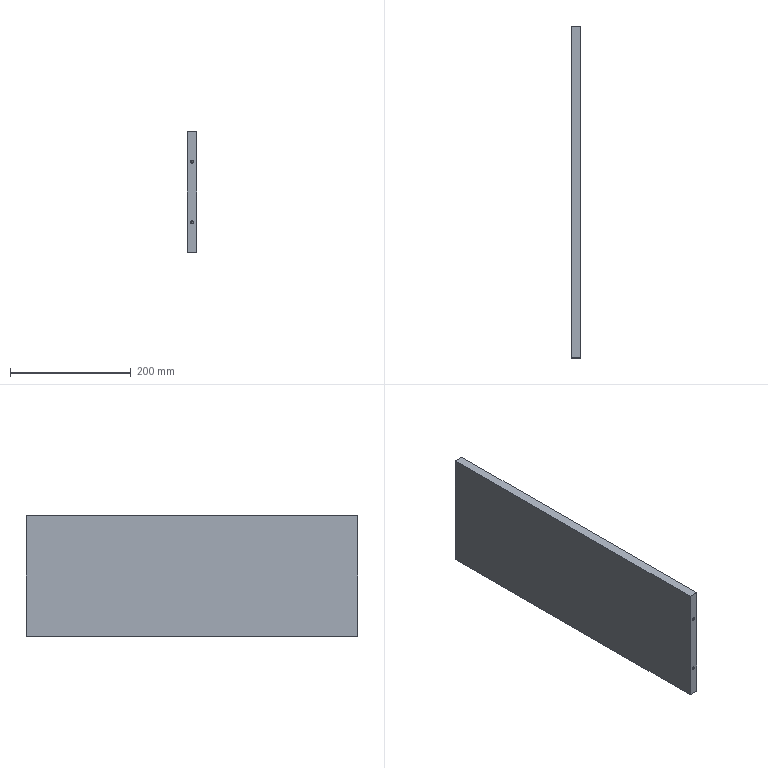Part | NX | features DATUM_CSYS 4, SIMPLE HOLE 4, SYMBOLIC_THREAD 4, SKETCH 3, EXTRACT_FACE 2, HOLE PACKAGE 2, EXTRUDE 1, Instance Feature 1, Mirror Feature 1 | 1 solid | 18 faces | box 15 x 550 x 200 mm | volume 1648864 mm3 | cone 8 | plane 6 | cylinder 4 | commonest cylinder face diameters 4.2 x4
STEP:
#1=CARTESIAN_POINT('',(-7.5,275.,0.));
#2=VERTEX_POINT('',#1);
#3=CARTESIAN_POINT('',(-7.5,-275.,0.));
#4=VERTEX_POINT('',#3);
#5=CARTESIAN_POINT('',(-7.5,275.,0.));
#6=DIRECTION('',(0.,-1.,0.));
#7=VECTOR('',#6,1000.);
#8=LINE('',#5,#7);
#9=EDGE_CURVE('',#2,#4,#8,.T.);
#10=ORIENTED_EDGE('',*,*,#9,.T.);
#11=CARTESIAN_POINT('',(-7.5,-275.,200.));
#12=VERTEX_POINT('',#11);
#13=CARTESIAN_POINT('',(-7.5,-275.,200.));
#14=DIRECTION('',(0.,0.,-1.));
#15=VECTOR('',#14,1000.);
#16=LINE('',#13,#15);
#17=EDGE_CURVE('',#12,#4,#16,.T.);
#18=ORIENTED_EDGE('',*,*,#17,.F.);
#19=CARTESIAN_POINT('',(-7.5,275.,200.));
#20=VERTEX_POINT('',#19);
#21=CARTESIAN_POINT('',(-7.5,275.,200.));
#22=DIRECTION('',(0.,-1.,0.));
#23=VECTOR('',#22,1000.);
#24=LINE('',#21,#23);
#25=EDGE_CURVE('',#20,#12,#24,.T.);
#26=ORIENTED_EDGE('',*,*,#25,.F.);
#27=CARTESIAN_POINT('',(-7.5,275.,200.));
#28=DIRECTION('',(0.,0.,-1.));
#29=VECTOR('',#28,1000.);
#30=LINE('',#27,#29);
#31=EDGE_CURVE('',#20,#2,#30,.T.);
#32=ORIENTED_EDGE('',*,*,#31,.T.);
#33=EDGE_LOOP('',(#10,#18,#26,#32));
#34=FACE_BOUND('',#33,.T.);
#35=CARTESIAN_POINT('',(-7.5,275.,200.));
#36=DIRECTION('',(1.,0.,0.));
#37=DIRECTION('',(0.,1.,0.));
#38=AXIS2_PLACEMENT_3D('',#35,#36,#37);
#39=PLANE('',#38);
#40=ADVANCED_FACE('',(#34),#39,.F.);
#41=CARTESIAN_POINT('',(0.,-275.,152.5));
#42=VERTEX_POINT('',#41);
#43=CARTESIAN_POINT('',(0.,-275.,150.));
#44=DIRECTION('',(0.,1.,0.));
#45=DIRECTION('',(0.,0.,1.));
#46=AXIS2_PLACEMENT_3D('',#43,#44,#45);
#47=CIRCLE('',#46,2.5);
#48=EDGE_CURVE('',#42,#42,#47,.T.);
#49=ORIENTED_EDGE('',*,*,#48,.T.);
#50=EDGE_LOOP('',(#49));
#51=FACE_BOUND('',#50,.T.);
#52=CARTESIAN_POINT('',(0.,-275.,52.5));
#53=VERTEX_POINT('',#52);
#54=CARTESIAN_POINT('',(0.,-275.,50.));
#55=DIRECTION('',(0.,1.,0.));
#56=DIRECTION('',(0.,0.,1.));
#57=AXIS2_PLACEMENT_3D('',#54,#55,#56);
#58=CIRCLE('',#57,2.5);
#59=EDGE_CURVE('',#53,#53,#58,.T.);
#60=ORIENTED_EDGE('',*,*,#59,.T.);
#61=EDGE_LOOP('',(#60));
#62=FACE_BOUND('',#61,.T.);
#63=CARTESIAN_POINT('',(7.5,-275.,0.));
#64=VERTEX_POINT('',#63);
#65=CARTESIAN_POINT('',(-7.5,-275.,0.));
#66=DIRECTION('',(1.,0.,0.));
#67=VECTOR('',#66,1000.);
#68=LINE('',#65,#67);
#69=EDGE_CURVE('',#4,#64,#68,.T.);
#70=ORIENTED_EDGE('',*,*,#69,.T.);
#71=CARTESIAN_POINT('',(7.5,-275.,200.));
#72=VERTEX_POINT('',#71);
#73=CARTESIAN_POINT('',(7.5,-275.,200.));
#74=DIRECTION('',(0.,0.,-1.));
#75=VECTOR('',#74,1000.);
#76=LINE('',#73,#75);
#77=EDGE_CURVE('',#72,#64,#76,.T.);
#78=ORIENTED_EDGE('',*,*,#77,.F.);
#79=CARTESIAN_POINT('',(-7.5,-275.,200.));
#80=DIRECTION('',(1.,0.,0.));
#81=VECTOR('',#80,1000.);
#82=LINE('',#79,#81);
#83=EDGE_CURVE('',#12,#72,#82,.T.);
#84=ORIENTED_EDGE('',*,*,#83,.F.);
#85=ORIENTED_EDGE('',*,*,#17,.T.);
#86=EDGE_LOOP('',(#70,#78,#84,#85));
#87=FACE_BOUND('',#86,.T.);
#88=CARTESIAN_POINT('',(-7.5,-275.,200.));
#89=DIRECTION('',(0.,1.,0.));
#90=DIRECTION('',(0.,0.,1.));
#91=AXIS2_PLACEMENT_3D('',#88,#89,#90);
#92=PLANE('',#91);
#93=ADVANCED_FACE('',(#51,#62,#87),#92,.F.);
#94=CARTESIAN_POINT('',(7.5,275.,0.));
#95=VERTEX_POINT('',#94);
#96=CARTESIAN_POINT('',(7.5,-275.,0.));
#97=DIRECTION('',(0.,1.,0.));
#98=VECTOR('',#97,1000.);
#99=LINE('',#96,#98);
#100=EDGE_CURVE('',#64,#95,#99,.T.);
#101=ORIENTED_EDGE('',*,*,#100,.T.);
#102=CARTESIAN_POINT('',(7.5,275.,200.));
#103=VERTEX_POINT('',#102);
#104=CARTESIAN_POINT('',(7.5,275.,200.));
#105=DIRECTION('',(0.,0.,-1.));
#106=VECTOR('',#105,1000.);
#107=LINE('',#104,#106);
#108=EDGE_CURVE('',#103,#95,#107,.T.);
#109=ORIENTED_EDGE('',*,*,#108,.F.);
#110=CARTESIAN_POINT('',(7.5,-275.,200.));
#111=DIRECTION('',(0.,1.,0.));
#112=VECTOR('',#111,1000.);
#113=LINE('',#110,#112);
#114=EDGE_CURVE('',#72,#103,#113,.T.);
#115=ORIENTED_EDGE('',*,*,#114,.F.);
#116=ORIENTED_EDGE('',*,*,#77,.T.);
#117=EDGE_LOOP('',(#101,#109,#115,#116));
#118=FACE_BOUND('',#117,.T.);
#119=CARTESIAN_POINT('',(7.5,-275.,200.));
#120=DIRECTION('',(-1.,0.,0.));
#121=DIRECTION('',(0.,-1.,0.));
#122=AXIS2_PLACEMENT_3D('',#119,#120,#121);
#123=PLANE('',#122);
#124=ADVANCED_FACE('',(#118),#123,.F.);
#125=CARTESIAN_POINT('',(0.,275.,147.5));
#126=VERTEX_POINT('',#125);
#127=CARTESIAN_POINT('',(0.,275.,150.));
#128=DIRECTION('',(0.,-1.,0.));
#129=DIRECTION('',(0.,0.,-1.));
#130=AXIS2_PLACEMENT_3D('',#127,#128,#129);
#131=CIRCLE('',#130,2.5);
#132=EDGE_CURVE('',#126,#126,#131,.T.);
#133=ORIENTED_EDGE('',*,*,#132,.T.);
#134=EDGE_LOOP('',(#133));
#135=FACE_BOUND('',#134,.T.);
#136=CARTESIAN_POINT('',(0.,275.,47.5));
#137=VERTEX_POINT('',#136);
#138=CARTESIAN_POINT('',(0.,275.,50.));
#139=DIRECTION('',(0.,-1.,0.));
#140=DIRECTION('',(0.,0.,-1.));
#141=AXIS2_PLACEMENT_3D('',#138,#139,#140);
#142=CIRCLE('',#141,2.5);
#143=EDGE_CURVE('',#137,#137,#142,.T.);
#144=ORIENTED_EDGE('',*,*,#143,.T.);
#145=EDGE_LOOP('',(#144));
#146=FACE_BOUND('',#145,.T.);
#147=CARTESIAN_POINT('',(7.5,275.,0.));
#148=DIRECTION('',(-1.,0.,0.));
#149=VECTOR('',#148,1000.);
#150=LINE('',#147,#149);
#151=EDGE_CURVE('',#95,#2,#150,.T.);
#152=ORIENTED_EDGE('',*,*,#151,.T.);
#153=ORIENTED_EDGE('',*,*,#31,.F.);
#154=CARTESIAN_POINT('',(7.5,275.,200.));
#155=DIRECTION('',(-1.,0.,0.));
#156=VECTOR('',#155,1000.);
#157=LINE('',#154,#156);
#158=EDGE_CURVE('',#103,#20,#157,.T.);
#159=ORIENTED_EDGE('',*,*,#158,.F.);
#160=ORIENTED_EDGE('',*,*,#108,.T.);
#161=EDGE_LOOP('',(#152,#153,#159,#160));
#162=FACE_BOUND('',#161,.T.);
#163=CARTESIAN_POINT('',(7.5,275.,200.));
#164=DIRECTION('',(0.,-1.,0.));
#165=DIRECTION('',(0.,0.,-1.));
#166=AXIS2_PLACEMENT_3D('',#163,#164,#165);
#167=PLANE('',#166);
#168=ADVANCED_FACE('',(#135,#146,#162),#167,.F.);
#169=ORIENTED_EDGE('',*,*,#25,.T.);
#170=ORIENTED_EDGE('',*,*,#83,.T.);
#171=ORIENTED_EDGE('',*,*,#114,.T.);
#172=ORIENTED_EDGE('',*,*,#158,.T.);
#173=EDGE_LOOP('',(#169,#170,#171,#172));
#174=FACE_BOUND('',#173,.T.);
#175=CARTESIAN_POINT('',(0.,0.,200.));
#176=DIRECTION('',(0.,0.,1.));
#177=DIRECTION('',(1.,0.,0.));
#178=AXIS2_PLACEMENT_3D('',#175,#176,#177);
#179=PLANE('',#178);
#180=ADVANCED_FACE('',(#174),#179,.T.);
#181=ORIENTED_EDGE('',*,*,#9,.F.);
#182=ORIENTED_EDGE('',*,*,#151,.F.);
#183=ORIENTED_EDGE('',*,*,#100,.F.);
#184=ORIENTED_EDGE('',*,*,#69,.F.);
#185=EDGE_LOOP('',(#181,#182,#183,#184));
#186=FACE_BOUND('',#185,.T.);
#187=CARTESIAN_POINT('',(0.,0.,0.));
#188=DIRECTION('',(0.,0.,1.));
#189=DIRECTION('',(1.,0.,0.));
#190=AXIS2_PLACEMENT_3D('',#187,#188,#189);
#191=PLANE('',#190);
#192=ADVANCED_FACE('',(#186),#191,.F.);
#193=CARTESIAN_POINT('',(0.,-255.,52.1));
#194=VERTEX_POINT('',#193);
#195=CARTESIAN_POINT('',(0.,-255.,50.));
#196=DIRECTION('',(0.,1.,0.));
#197=DIRECTION('',(0.,0.,1.));
#198=AXIS2_PLACEMENT_3D('',#195,#196,#197);
#199=CIRCLE('',#198,2.1);
#200=EDGE_CURVE('',#194,#194,#199,.F.);
#201=ORIENTED_EDGE('',*,*,#200,.T.);
#202=EDGE_LOOP('',(#201));
#203=FACE_BOUND('',#202,.T.);
#204=CARTESIAN_POINT('',(0.,-253.738,50.));
#205=VERTEX_POINT('',#204);
#206=VERTEX_LOOP('',#205);
#207=FACE_BOUND('',#206,.T.);
#208=CARTESIAN_POINT('',(0.,-255.,50.));
#209=DIRECTION('',(0.,-1.,0.));
#210=DIRECTION('',(0.,0.,-1.));
#211=AXIS2_PLACEMENT_3D('',#208,#209,#210);
#212=CONICAL_SURFACE('',#211,2.1,1.03);
#213=ADVANCED_FACE('',(#203,#207),#212,.F.);
#214=CARTESIAN_POINT('',(0.,-274.6,52.1));
#215=VERTEX_POINT('',#214);
#216=CARTESIAN_POINT('',(0.,-274.6,50.));
#217=DIRECTION('',(0.,1.,0.));
#218=DIRECTION('',(0.,0.,1.));
#219=AXIS2_PLACEMENT_3D('',#216,#217,#218);
#220=CIRCLE('',#219,2.1);
#221=EDGE_CURVE('',#215,#215,#220,.F.);
#222=ORIENTED_EDGE('',*,*,#221,.T.);
#223=EDGE_LOOP('',(#222));
#224=FACE_BOUND('',#223,.T.);
#225=ORIENTED_EDGE('',*,*,#200,.F.);
#226=EDGE_LOOP('',(#225));
#227=FACE_BOUND('',#226,.T.);
#228=CARTESIAN_POINT('',(0.,-275.,50.));
#229=DIRECTION('',(0.,1.,0.));
#230=DIRECTION('',(0.,0.,1.));
#231=AXIS2_PLACEMENT_3D('',#228,#229,#230);
#232=CYLINDRICAL_SURFACE('',#231,2.1);
#233=ADVANCED_FACE('',(#224,#227),#232,.F.);
#234=ORIENTED_EDGE('',*,*,#221,.F.);
#235=EDGE_LOOP('',(#234));
#236=FACE_BOUND('',#235,.T.);
#237=ORIENTED_EDGE('',*,*,#59,.F.);
#238=EDGE_LOOP('',(#237));
#239=FACE_BOUND('',#238,.T.);
#240=CARTESIAN_POINT('',(0.,-275.,50.));
#241=DIRECTION('',(0.,-1.,0.));
#242=DIRECTION('',(0.,0.,-1.));
#243=AXIS2_PLACEMENT_3D('',#240,#241,#242);
#244=CONICAL_SURFACE('',#243,2.5,0.7854);
#245=ADVANCED_FACE('',(#236,#239),#244,.F.);
#246=CARTESIAN_POINT('',(0.,-255.,152.1));
#247=VERTEX_POINT('',#246);
#248=CARTESIAN_POINT('',(0.,-255.,150.));
#249=DIRECTION('',(0.,1.,0.));
#250=DIRECTION('',(0.,0.,1.));
#251=AXIS2_PLACEMENT_3D('',#248,#249,#250);
#252=CIRCLE('',#251,2.1);
#253=EDGE_CURVE('',#247,#247,#252,.F.);
#254=ORIENTED_EDGE('',*,*,#253,.T.);
#255=EDGE_LOOP('',(#254));
#256=FACE_BOUND('',#255,.T.);
#257=CARTESIAN_POINT('',(0.,-253.738,150.));
#258=VERTEX_POINT('',#257);
#259=VERTEX_LOOP('',#258);
#260=FACE_BOUND('',#259,.T.);
#261=CARTESIAN_POINT('',(0.,-255.,150.));
#262=DIRECTION('',(0.,-1.,0.));
#263=DIRECTION('',(0.,0.,-1.));
#264=AXIS2_PLACEMENT_3D('',#261,#262,#263);
#265=CONICAL_SURFACE('',#264,2.1,1.03);
#266=ADVANCED_FACE('',(#256,#260),#265,.F.);
#267=CARTESIAN_POINT('',(0.,-274.6,152.1));
#268=VERTEX_POINT('',#267);
#269=CARTESIAN_POINT('',(0.,-274.6,150.));
#270=DIRECTION('',(0.,1.,0.));
#271=DIRECTION('',(0.,0.,1.));
#272=AXIS2_PLACEMENT_3D('',#269,#270,#271);
#273=CIRCLE('',#272,2.1);
#274=EDGE_CURVE('',#268,#268,#273,.F.);
#275=ORIENTED_EDGE('',*,*,#274,.T.);
#276=EDGE_LOOP('',(#275));
#277=FACE_BOUND('',#276,.T.);
#278=ORIENTED_EDGE('',*,*,#253,.F.);
#279=EDGE_LOOP('',(#278));
#280=FACE_BOUND('',#279,.T.);
#281=CARTESIAN_POINT('',(0.,-275.,150.));
#282=DIRECTION('',(0.,1.,0.));
#283=DIRECTION('',(0.,0.,1.));
#284=AXIS2_PLACEMENT_3D('',#281,#282,#283);
#285=CYLINDRICAL_SURFACE('',#284,2.1);
#286=ADVANCED_FACE('',(#277,#280),#285,.F.);
#287=ORIENTED_EDGE('',*,*,#274,.F.);
#288=EDGE_LOOP('',(#287));
#289=FACE_BOUND('',#288,.T.);
#290=ORIENTED_EDGE('',*,*,#48,.F.);
#291=EDGE_LOOP('',(#290));
#292=FACE_BOUND('',#291,.T.);
#293=CARTESIAN_POINT('',(0.,-275.,150.));
#294=DIRECTION('',(0.,-1.,0.));
#295=DIRECTION('',(0.,0.,-1.));
#296=AXIS2_PLACEMENT_3D('',#293,#294,#295);
#297=CONICAL_SURFACE('',#296,2.5,0.7854);
#298=ADVANCED_FACE('',(#289,#292),#297,.F.);
#299=CARTESIAN_POINT('',(0.,255.,47.9));
#300=VERTEX_POINT('',#299);
#301=CARTESIAN_POINT('',(0.,255.,50.));
#302=DIRECTION('',(0.,-1.,0.));
#303=DIRECTION('',(0.,0.,-1.));
#304=AXIS2_PLACEMENT_3D('',#301,#302,#303);
#305=CIRCLE('',#304,2.1);
#306=EDGE_CURVE('',#300,#300,#305,.T.);
#307=ORIENTED_EDGE('',*,*,#306,.F.);
#308=EDGE_LOOP('',(#307));
#309=FACE_BOUND('',#308,.T.);
#310=CARTESIAN_POINT('',(0.,253.738,50.));
#311=VERTEX_POINT('',#310);
#312=VERTEX_LOOP('',#311);
#313=FACE_BOUND('',#312,.T.);
#314=CARTESIAN_POINT('',(0.,255.,50.));
#315=DIRECTION('',(0.,1.,0.));
#316=DIRECTION('',(0.,0.,1.));
#317=AXIS2_PLACEMENT_3D('',#314,#315,#316);
#318=CONICAL_SURFACE('',#317,2.1,1.03);
#319=ADVANCED_FACE('',(#309,#313),#318,.F.);
#320=CARTESIAN_POINT('',(0.,274.6,47.9));
#321=VERTEX_POINT('',#320);
#322=CARTESIAN_POINT('',(0.,274.6,50.));
#323=DIRECTION('',(0.,-1.,0.));
#324=DIRECTION('',(0.,0.,-1.));
#325=AXIS2_PLACEMENT_3D('',#322,#323,#324);
#326=CIRCLE('',#325,2.1);
#327=EDGE_CURVE('',#321,#321,#326,.T.);
#328=ORIENTED_EDGE('',*,*,#327,.F.);
#329=EDGE_LOOP('',(#328));
#330=FACE_BOUND('',#329,.T.);
#331=ORIENTED_EDGE('',*,*,#306,.T.);
#332=EDGE_LOOP('',(#331));
#333=FACE_BOUND('',#332,.T.);
#334=CARTESIAN_POINT('',(0.,275.,50.));
#335=DIRECTION('',(0.,-1.,0.));
#336=DIRECTION('',(0.,0.,-1.));
#337=AXIS2_PLACEMENT_3D('',#334,#335,#336);
#338=CYLINDRICAL_SURFACE('',#337,2.1);
#339=ADVANCED_FACE('',(#330,#333),#338,.F.);
#340=ORIENTED_EDGE('',*,*,#327,.T.);
#341=EDGE_LOOP('',(#340));
#342=FACE_BOUND('',#341,.T.);
#343=ORIENTED_EDGE('',*,*,#143,.F.);
#344=EDGE_LOOP('',(#343));
#345=FACE_BOUND('',#344,.T.);
#346=CARTESIAN_POINT('',(0.,275.,50.));
#347=DIRECTION('',(0.,1.,0.));
#348=DIRECTION('',(0.,0.,1.));
#349=AXIS2_PLACEMENT_3D('',#346,#347,#348);
#350=CONICAL_SURFACE('',#349,2.5,0.7854);
#351=ADVANCED_FACE('',(#342,#345),#350,.F.);
#352=CARTESIAN_POINT('',(0.,255.,147.9));
#353=VERTEX_POINT('',#352);
#354=CARTESIAN_POINT('',(0.,255.,150.));
#355=DIRECTION('',(0.,-1.,0.));
#356=DIRECTION('',(0.,0.,-1.));
#357=AXIS2_PLACEMENT_3D('',#354,#355,#356);
#358=CIRCLE('',#357,2.1);
#359=EDGE_CURVE('',#353,#353,#358,.T.);
#360=ORIENTED_EDGE('',*,*,#359,.F.);
#361=EDGE_LOOP('',(#360));
#362=FACE_BOUND('',#361,.T.);
#363=CARTESIAN_POINT('',(0.,253.738,150.));
#364=VERTEX_POINT('',#363);
#365=VERTEX_LOOP('',#364);
#366=FACE_BOUND('',#365,.T.);
#367=CARTESIAN_POINT('',(0.,255.,150.));
#368=DIRECTION('',(0.,1.,0.));
#369=DIRECTION('',(0.,0.,1.));
#370=AXIS2_PLACEMENT_3D('',#367,#368,#369);
#371=CONICAL_SURFACE('',#370,2.1,1.03);
#372=ADVANCED_FACE('',(#362,#366),#371,.F.);
#373=CARTESIAN_POINT('',(0.,274.6,147.9));
#374=VERTEX_POINT('',#373);
#375=CARTESIAN_POINT('',(0.,274.6,150.));
#376=DIRECTION('',(0.,-1.,0.));
#377=DIRECTION('',(0.,0.,-1.));
#378=AXIS2_PLACEMENT_3D('',#375,#376,#377);
#379=CIRCLE('',#378,2.1);
#380=EDGE_CURVE('',#374,#374,#379,.T.);
#381=ORIENTED_EDGE('',*,*,#380,.F.);
#382=EDGE_LOOP('',(#381));
#383=FACE_BOUND('',#382,.T.);
#384=ORIENTED_EDGE('',*,*,#359,.T.);
#385=EDGE_LOOP('',(#384));
#386=FACE_BOUND('',#385,.T.);
#387=CARTESIAN_POINT('',(0.,275.,150.));
#388=DIRECTION('',(0.,-1.,0.));
#389=DIRECTION('',(0.,0.,-1.));
#390=AXIS2_PLACEMENT_3D('',#387,#388,#389);
#391=CYLINDRICAL_SURFACE('',#390,2.1);
#392=ADVANCED_FACE('',(#383,#386),#391,.F.);
#393=ORIENTED_EDGE('',*,*,#380,.T.);
#394=EDGE_LOOP('',(#393));
#395=FACE_BOUND('',#394,.T.);
#396=ORIENTED_EDGE('',*,*,#132,.F.);
#397=EDGE_LOOP('',(#396));
#398=FACE_BOUND('',#397,.T.);
#399=CARTESIAN_POINT('',(0.,275.,150.));
#400=DIRECTION('',(0.,1.,0.));
#401=DIRECTION('',(0.,0.,1.));
#402=AXIS2_PLACEMENT_3D('',#399,#400,#401);
#403=CONICAL_SURFACE('',#402,2.5,0.7854);
#404=ADVANCED_FACE('',(#395,#398),#403,.F.);
#405=CLOSED_SHELL('',(#40,#93,#124,#168,#180,#192,#213,#233,#245,#266,#286,#298,#319,#339,#351,#372,#392,#404));
#406=MANIFOLD_SOLID_BREP('',#405);
#407=(LENGTH_UNIT()NAMED_UNIT(*)SI_UNIT(.MILLI.,.METRE.));
#408=UNCERTAINTY_MEASURE_WITH_UNIT(LENGTH_MEASURE(0.00001),#407,'','');
#409=(NAMED_UNIT(*)PLANE_ANGLE_UNIT()SI_UNIT($,.RADIAN.));
#410=(NAMED_UNIT(*)SI_UNIT($,.STERADIAN.)SOLID_ANGLE_UNIT());
#411=(GEOMETRIC_REPRESENTATION_CONTEXT(3)GLOBAL_UNCERTAINTY_ASSIGNED_CONTEXT((#408))GLOBAL_UNIT_ASSIGNED_CONTEXT((#407,#409,#410))REPRESENTATION_CONTEXT('',''));
#412=ADVANCED_BREP_SHAPE_REPRESENTATION('',(#406),#411);